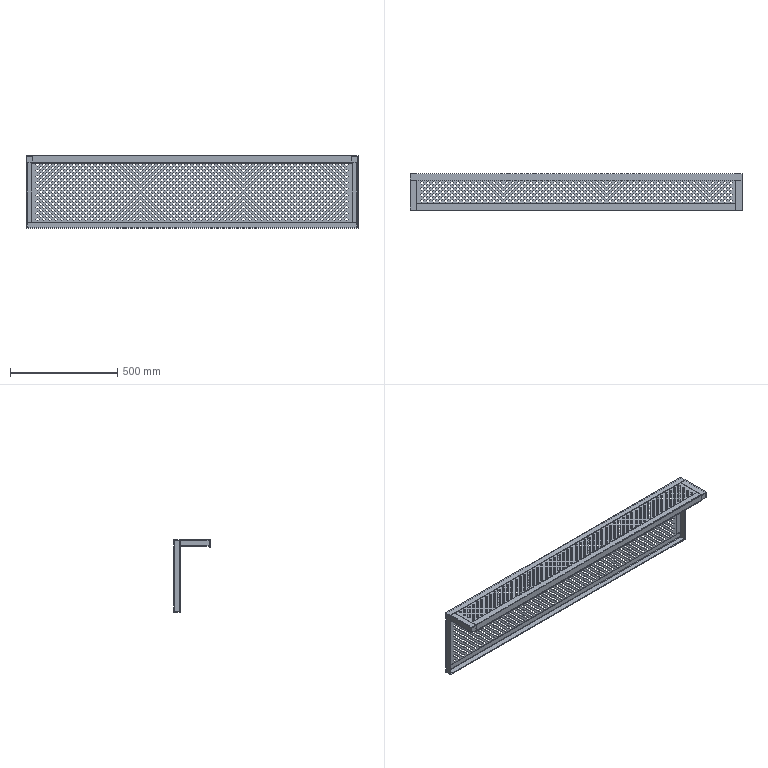Part | SolidWorks | features BaseBody 11 | 11 solids | 5481 faces | volume 1424009 mm3 | plane 5448 | cylinder 33 | commonest cylinder face diameters 4 x33